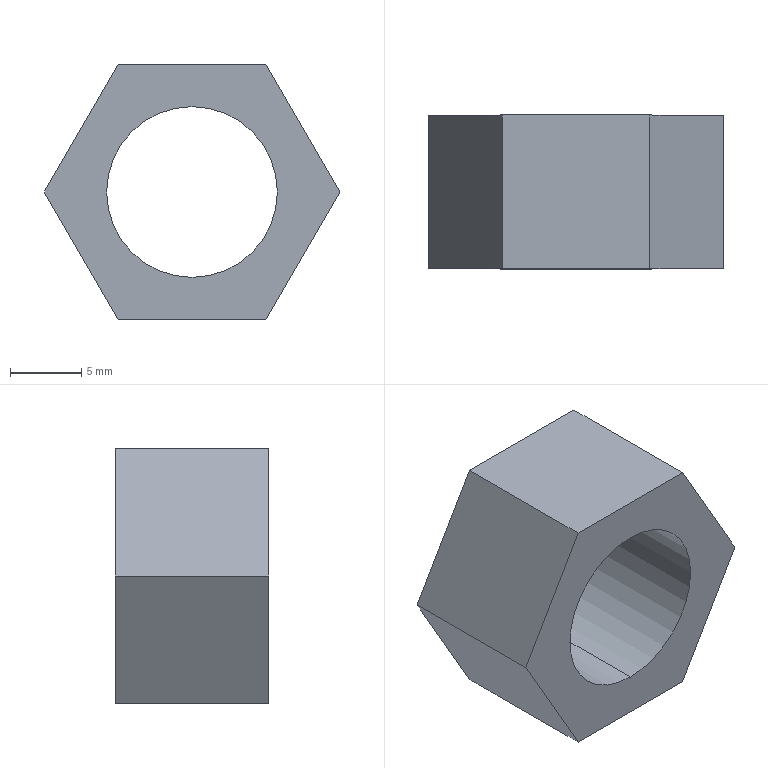Part | STEP file | Pin shaft nut M12 | 1 solid | 10 faces | box 20.785 x 10.8 x 18 mm | volume 1809 mm3 | plane 8 | cylinder 2 | commonest cylinder face diameters 12 x2
STEP:
#1=CARTESIAN_POINT('',(0.,10.8,-6.));
#2=VERTEX_POINT('',#1);
#3=CARTESIAN_POINT('',(0.,10.8,6.));
#4=VERTEX_POINT('',#3);
#5=CARTESIAN_POINT('',(0.,10.8,0.));
#6=DIRECTION('',(0.,1.,0.));
#7=DIRECTION('',(0.,0.,1.));
#8=AXIS2_PLACEMENT_3D('',#5,#6,#7);
#9=CIRCLE('',#8,6.);
#10=EDGE_CURVE('',#2,#4,#9,.T.);
#11=ORIENTED_EDGE('',*,*,#10,.T.);
#12=CARTESIAN_POINT('',(0.,0.,6.));
#13=VERTEX_POINT('',#12);
#14=CARTESIAN_POINT('',(0.,10.8,6.));
#15=DIRECTION('',(0.,-1.,0.));
#16=VECTOR('',#15,1000.);
#17=LINE('',#14,#16);
#18=EDGE_CURVE('',#4,#13,#17,.T.);
#19=ORIENTED_EDGE('',*,*,#18,.T.);
#20=CARTESIAN_POINT('',(0.,0.,-6.));
#21=VERTEX_POINT('',#20);
#22=CARTESIAN_POINT('',(0.,0.,0.));
#23=DIRECTION('',(0.,1.,0.));
#24=DIRECTION('',(0.,0.,1.));
#25=AXIS2_PLACEMENT_3D('',#22,#23,#24);
#26=CIRCLE('',#25,6.);
#27=EDGE_CURVE('',#21,#13,#26,.T.);
#28=ORIENTED_EDGE('',*,*,#27,.F.);
#29=CARTESIAN_POINT('',(0.,10.8,-6.));
#30=DIRECTION('',(0.,-1.,0.));
#31=VECTOR('',#30,1000.);
#32=LINE('',#29,#31);
#33=EDGE_CURVE('',#2,#21,#32,.T.);
#34=ORIENTED_EDGE('',*,*,#33,.F.);
#35=EDGE_LOOP('',(#11,#19,#28,#34));
#36=FACE_OUTER_BOUND('',#35,.T.);
#37=CARTESIAN_POINT('',(0.,10.8,0.));
#38=DIRECTION('',(0.,-1.,0.));
#39=DIRECTION('',(0.,0.,-1.));
#40=AXIS2_PLACEMENT_3D('',#37,#38,#39);
#41=CYLINDRICAL_SURFACE('',#40,6.);
#42=ADVANCED_FACE('',(#36),#41,.F.);
#43=CARTESIAN_POINT('',(-10.392,0.,0.));
#44=VERTEX_POINT('',#43);
#45=CARTESIAN_POINT('',(-5.196,0.,-9.));
#46=VERTEX_POINT('',#45);
#47=CARTESIAN_POINT('',(-7.794,0.,-4.5));
#48=DIRECTION('',(0.5,0.,-0.866));
#49=VECTOR('',#48,1000.);
#50=LINE('',#47,#49);
#51=EDGE_CURVE('',#44,#46,#50,.T.);
#52=ORIENTED_EDGE('',*,*,#51,.F.);
#53=CARTESIAN_POINT('',(-10.392,10.8,0.));
#54=VERTEX_POINT('',#53);
#55=CARTESIAN_POINT('',(-10.392,10.8,0.));
#56=DIRECTION('',(0.,-1.,0.));
#57=VECTOR('',#56,1000.);
#58=LINE('',#55,#57);
#59=EDGE_CURVE('',#54,#44,#58,.T.);
#60=ORIENTED_EDGE('',*,*,#59,.F.);
#61=CARTESIAN_POINT('',(-5.196,10.8,-9.));
#62=VERTEX_POINT('',#61);
#63=CARTESIAN_POINT('',(-7.794,10.8,-4.5));
#64=DIRECTION('',(0.5,0.,-0.866));
#65=VECTOR('',#64,1000.);
#66=LINE('',#63,#65);
#67=EDGE_CURVE('',#54,#62,#66,.T.);
#68=ORIENTED_EDGE('',*,*,#67,.T.);
#69=CARTESIAN_POINT('',(-5.196,10.8,-9.));
#70=DIRECTION('',(0.,-1.,0.));
#71=VECTOR('',#70,1000.);
#72=LINE('',#69,#71);
#73=EDGE_CURVE('',#62,#46,#72,.T.);
#74=ORIENTED_EDGE('',*,*,#73,.T.);
#75=EDGE_LOOP('',(#52,#60,#68,#74));
#76=FACE_OUTER_BOUND('',#75,.T.);
#77=CARTESIAN_POINT('',(-7.794,10.8,-4.5));
#78=DIRECTION('',(-0.866,0.,-0.5));
#79=DIRECTION('',(-0.5,0.,0.866));
#80=AXIS2_PLACEMENT_3D('',#77,#78,#79);
#81=PLANE('',#80);
#82=ADVANCED_FACE('',(#76),#81,.T.);
#83=CARTESIAN_POINT('',(-5.196,0.,9.));
#84=VERTEX_POINT('',#83);
#85=CARTESIAN_POINT('',(-7.794,0.,4.5));
#86=DIRECTION('',(-0.5,0.,-0.866));
#87=VECTOR('',#86,1000.);
#88=LINE('',#85,#87);
#89=EDGE_CURVE('',#84,#44,#88,.T.);
#90=ORIENTED_EDGE('',*,*,#89,.F.);
#91=CARTESIAN_POINT('',(-5.196,10.8,9.));
#92=VERTEX_POINT('',#91);
#93=CARTESIAN_POINT('',(-5.196,10.8,9.));
#94=DIRECTION('',(0.,-1.,0.));
#95=VECTOR('',#94,1000.);
#96=LINE('',#93,#95);
#97=EDGE_CURVE('',#92,#84,#96,.T.);
#98=ORIENTED_EDGE('',*,*,#97,.F.);
#99=CARTESIAN_POINT('',(-7.794,10.8,4.5));
#100=DIRECTION('',(-0.5,0.,-0.866));
#101=VECTOR('',#100,1000.);
#102=LINE('',#99,#101);
#103=EDGE_CURVE('',#92,#54,#102,.T.);
#104=ORIENTED_EDGE('',*,*,#103,.T.);
#105=ORIENTED_EDGE('',*,*,#59,.T.);
#106=EDGE_LOOP('',(#90,#98,#104,#105));
#107=FACE_OUTER_BOUND('',#106,.T.);
#108=CARTESIAN_POINT('',(-7.794,10.8,4.5));
#109=DIRECTION('',(-0.866,0.,0.5));
#110=DIRECTION('',(0.5,0.,0.866));
#111=AXIS2_PLACEMENT_3D('',#108,#109,#110);
#112=PLANE('',#111);
#113=ADVANCED_FACE('',(#107),#112,.T.);
#114=CARTESIAN_POINT('',(5.196,0.,9.));
#115=VERTEX_POINT('',#114);
#116=CARTESIAN_POINT('',(0.,0.,9.));
#117=DIRECTION('',(-1.,0.,0.));
#118=VECTOR('',#117,1000.);
#119=LINE('',#116,#118);
#120=EDGE_CURVE('',#115,#84,#119,.T.);
#121=ORIENTED_EDGE('',*,*,#120,.F.);
#122=CARTESIAN_POINT('',(5.196,10.8,9.));
#123=VERTEX_POINT('',#122);
#124=CARTESIAN_POINT('',(5.196,10.8,9.));
#125=DIRECTION('',(0.,-1.,0.));
#126=VECTOR('',#125,1000.);
#127=LINE('',#124,#126);
#128=EDGE_CURVE('',#123,#115,#127,.T.);
#129=ORIENTED_EDGE('',*,*,#128,.F.);
#130=CARTESIAN_POINT('',(0.,10.8,9.));
#131=DIRECTION('',(-1.,0.,0.));
#132=VECTOR('',#131,1000.);
#133=LINE('',#130,#132);
#134=EDGE_CURVE('',#123,#92,#133,.T.);
#135=ORIENTED_EDGE('',*,*,#134,.T.);
#136=ORIENTED_EDGE('',*,*,#97,.T.);
#137=EDGE_LOOP('',(#121,#129,#135,#136));
#138=FACE_OUTER_BOUND('',#137,.T.);
#139=CARTESIAN_POINT('',(0.,10.8,9.));
#140=DIRECTION('',(0.,0.,1.));
#141=DIRECTION('',(1.,0.,0.));
#142=AXIS2_PLACEMENT_3D('',#139,#140,#141);
#143=PLANE('',#142);
#144=ADVANCED_FACE('',(#138),#143,.T.);
#145=CARTESIAN_POINT('',(10.392,0.,0.));
#146=VERTEX_POINT('',#145);
#147=CARTESIAN_POINT('',(7.794,0.,4.5));
#148=DIRECTION('',(-0.5,0.,0.866));
#149=VECTOR('',#148,1000.);
#150=LINE('',#147,#149);
#151=EDGE_CURVE('',#146,#115,#150,.T.);
#152=ORIENTED_EDGE('',*,*,#151,.F.);
#153=CARTESIAN_POINT('',(10.392,10.8,0.));
#154=VERTEX_POINT('',#153);
#155=CARTESIAN_POINT('',(10.392,10.8,0.));
#156=DIRECTION('',(0.,-1.,0.));
#157=VECTOR('',#156,1000.);
#158=LINE('',#155,#157);
#159=EDGE_CURVE('',#154,#146,#158,.T.);
#160=ORIENTED_EDGE('',*,*,#159,.F.);
#161=CARTESIAN_POINT('',(7.794,10.8,4.5));
#162=DIRECTION('',(-0.5,0.,0.866));
#163=VECTOR('',#162,1000.);
#164=LINE('',#161,#163);
#165=EDGE_CURVE('',#154,#123,#164,.T.);
#166=ORIENTED_EDGE('',*,*,#165,.T.);
#167=ORIENTED_EDGE('',*,*,#128,.T.);
#168=EDGE_LOOP('',(#152,#160,#166,#167));
#169=FACE_OUTER_BOUND('',#168,.T.);
#170=CARTESIAN_POINT('',(7.794,10.8,4.5));
#171=DIRECTION('',(0.866,0.,0.5));
#172=DIRECTION('',(0.5,0.,-0.866));
#173=AXIS2_PLACEMENT_3D('',#170,#171,#172);
#174=PLANE('',#173);
#175=ADVANCED_FACE('',(#169),#174,.T.);
#176=CARTESIAN_POINT('',(5.196,0.,-9.));
#177=VERTEX_POINT('',#176);
#178=CARTESIAN_POINT('',(7.794,0.,-4.5));
#179=DIRECTION('',(0.5,0.,0.866));
#180=VECTOR('',#179,1000.);
#181=LINE('',#178,#180);
#182=EDGE_CURVE('',#177,#146,#181,.T.);
#183=ORIENTED_EDGE('',*,*,#182,.F.);
#184=CARTESIAN_POINT('',(5.196,10.8,-9.));
#185=VERTEX_POINT('',#184);
#186=CARTESIAN_POINT('',(5.196,10.8,-9.));
#187=DIRECTION('',(0.,-1.,0.));
#188=VECTOR('',#187,1000.);
#189=LINE('',#186,#188);
#190=EDGE_CURVE('',#185,#177,#189,.T.);
#191=ORIENTED_EDGE('',*,*,#190,.F.);
#192=CARTESIAN_POINT('',(7.794,10.8,-4.5));
#193=DIRECTION('',(0.5,0.,0.866));
#194=VECTOR('',#193,1000.);
#195=LINE('',#192,#194);
#196=EDGE_CURVE('',#185,#154,#195,.T.);
#197=ORIENTED_EDGE('',*,*,#196,.T.);
#198=ORIENTED_EDGE('',*,*,#159,.T.);
#199=EDGE_LOOP('',(#183,#191,#197,#198));
#200=FACE_OUTER_BOUND('',#199,.T.);
#201=CARTESIAN_POINT('',(7.794,10.8,-4.5));
#202=DIRECTION('',(0.866,0.,-0.5));
#203=DIRECTION('',(-0.5,0.,-0.866));
#204=AXIS2_PLACEMENT_3D('',#201,#202,#203);
#205=PLANE('',#204);
#206=ADVANCED_FACE('',(#200),#205,.T.);
#207=CARTESIAN_POINT('',(0.,0.,-9.));
#208=DIRECTION('',(1.,0.,0.));
#209=VECTOR('',#208,1000.);
#210=LINE('',#207,#209);
#211=EDGE_CURVE('',#46,#177,#210,.T.);
#212=ORIENTED_EDGE('',*,*,#211,.F.);
#213=ORIENTED_EDGE('',*,*,#73,.F.);
#214=CARTESIAN_POINT('',(0.,10.8,-9.));
#215=DIRECTION('',(1.,0.,0.));
#216=VECTOR('',#215,1000.);
#217=LINE('',#214,#216);
#218=EDGE_CURVE('',#62,#185,#217,.T.);
#219=ORIENTED_EDGE('',*,*,#218,.T.);
#220=ORIENTED_EDGE('',*,*,#190,.T.);
#221=EDGE_LOOP('',(#212,#213,#219,#220));
#222=FACE_OUTER_BOUND('',#221,.T.);
#223=CARTESIAN_POINT('',(0.,10.8,-9.));
#224=DIRECTION('',(0.,0.,-1.));
#225=DIRECTION('',(-1.,0.,0.));
#226=AXIS2_PLACEMENT_3D('',#223,#224,#225);
#227=PLANE('',#226);
#228=ADVANCED_FACE('',(#222),#227,.T.);
#229=ORIENTED_EDGE('',*,*,#10,.F.);
#230=CARTESIAN_POINT('',(0.,10.8,0.));
#231=DIRECTION('',(0.,1.,0.));
#232=DIRECTION('',(0.,0.,1.));
#233=AXIS2_PLACEMENT_3D('',#230,#231,#232);
#234=CIRCLE('',#233,6.);
#235=EDGE_CURVE('',#4,#2,#234,.T.);
#236=ORIENTED_EDGE('',*,*,#235,.F.);
#237=EDGE_LOOP('',(#229,#236));
#238=FACE_BOUND('',#237,.T.);
#239=ORIENTED_EDGE('',*,*,#67,.F.);
#240=ORIENTED_EDGE('',*,*,#103,.F.);
#241=ORIENTED_EDGE('',*,*,#134,.F.);
#242=ORIENTED_EDGE('',*,*,#165,.F.);
#243=ORIENTED_EDGE('',*,*,#196,.F.);
#244=ORIENTED_EDGE('',*,*,#218,.F.);
#245=EDGE_LOOP('',(#239,#240,#241,#242,#243,#244));
#246=FACE_OUTER_BOUND('',#245,.T.);
#247=CARTESIAN_POINT('',(0.,10.8,0.));
#248=DIRECTION('',(0.,1.,0.));
#249=DIRECTION('',(0.,0.,1.));
#250=AXIS2_PLACEMENT_3D('',#247,#248,#249);
#251=PLANE('',#250);
#252=ADVANCED_FACE('',(#238,#246),#251,.T.);
#253=ORIENTED_EDGE('',*,*,#27,.T.);
#254=CARTESIAN_POINT('',(0.,0.,0.));
#255=DIRECTION('',(0.,1.,0.));
#256=DIRECTION('',(0.,0.,1.));
#257=AXIS2_PLACEMENT_3D('',#254,#255,#256);
#258=CIRCLE('',#257,6.);
#259=EDGE_CURVE('',#13,#21,#258,.T.);
#260=ORIENTED_EDGE('',*,*,#259,.T.);
#261=EDGE_LOOP('',(#253,#260));
#262=FACE_BOUND('',#261,.T.);
#263=ORIENTED_EDGE('',*,*,#51,.T.);
#264=ORIENTED_EDGE('',*,*,#211,.T.);
#265=ORIENTED_EDGE('',*,*,#182,.T.);
#266=ORIENTED_EDGE('',*,*,#151,.T.);
#267=ORIENTED_EDGE('',*,*,#120,.T.);
#268=ORIENTED_EDGE('',*,*,#89,.T.);
#269=EDGE_LOOP('',(#263,#264,#265,#266,#267,#268));
#270=FACE_OUTER_BOUND('',#269,.T.);
#271=CARTESIAN_POINT('',(0.,0.,0.));
#272=DIRECTION('',(0.,1.,0.));
#273=DIRECTION('',(0.,0.,1.));
#274=AXIS2_PLACEMENT_3D('',#271,#272,#273);
#275=PLANE('',#274);
#276=ADVANCED_FACE('',(#262,#270),#275,.F.);
#277=ORIENTED_EDGE('',*,*,#18,.F.);
#278=ORIENTED_EDGE('',*,*,#235,.T.);
#279=ORIENTED_EDGE('',*,*,#33,.T.);
#280=ORIENTED_EDGE('',*,*,#259,.F.);
#281=EDGE_LOOP('',(#277,#278,#279,#280));
#282=FACE_OUTER_BOUND('',#281,.T.);
#283=CARTESIAN_POINT('',(0.,10.8,0.));
#284=DIRECTION('',(0.,-1.,0.));
#285=DIRECTION('',(0.,0.,-1.));
#286=AXIS2_PLACEMENT_3D('',#283,#284,#285);
#287=CYLINDRICAL_SURFACE('',#286,6.);
#288=ADVANCED_FACE('',(#282),#287,.F.);
#289=CLOSED_SHELL('',(#42,#82,#113,#144,#175,#206,#228,#252,#276,#288));
#290=MANIFOLD_SOLID_BREP('',#289);
#291=CARTESIAN_POINT('',(0.,0.,0.));
#292=DIRECTION('',(0.,0.,1.));
#293=DIRECTION('',(1.,0.,0.));
#294=AXIS2_PLACEMENT_3D('',#291,#292,#293);
#295=(LENGTH_UNIT()NAMED_UNIT(*)SI_UNIT(.MILLI.,.METRE.));
#296=UNCERTAINTY_MEASURE_WITH_UNIT(LENGTH_MEASURE(0.00001),#295,'','');
#297=(NAMED_UNIT(*)PLANE_ANGLE_UNIT()SI_UNIT($,.RADIAN.));
#298=(NAMED_UNIT(*)SI_UNIT($,.STERADIAN.)SOLID_ANGLE_UNIT());
#299=(GEOMETRIC_REPRESENTATION_CONTEXT(3)GLOBAL_UNCERTAINTY_ASSIGNED_CONTEXT((#296))GLOBAL_UNIT_ASSIGNED_CONTEXT((#295,#297,#298))REPRESENTATION_CONTEXT('',''));
#300=ADVANCED_BREP_SHAPE_REPRESENTATION('',(#290,#294),#299);